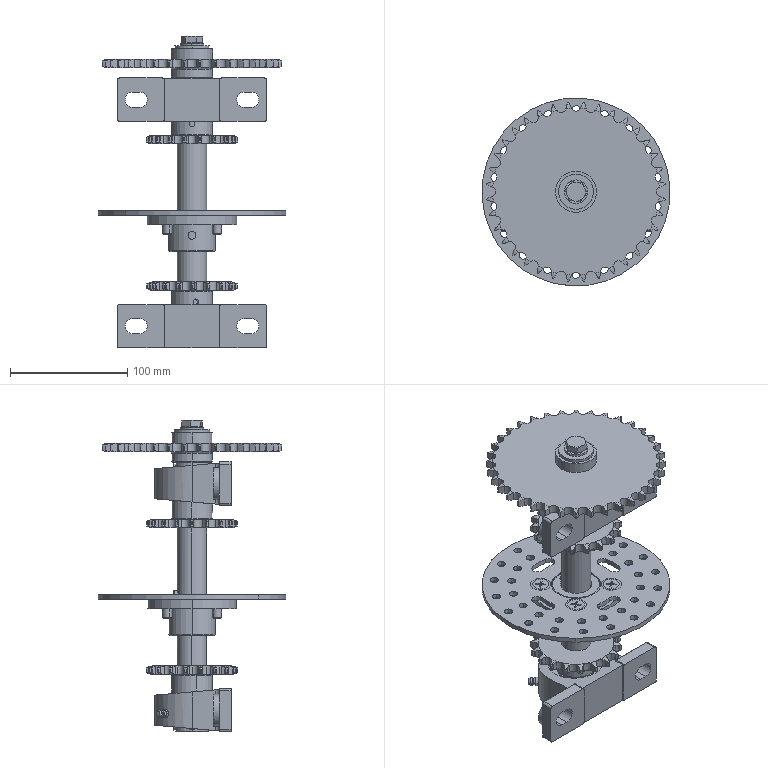Part | SolidWorks | 24 solids | 1345 faces | box 160 x 160 x 265.6 mm | volume 650641 mm3 | cylinder 702 | plane 320 | torus 200 | cone 123 | commonest cylinder face diameters 7 x76 12.41 x72 22.269 x72 77.611 x72 8.653 x48 78 x38